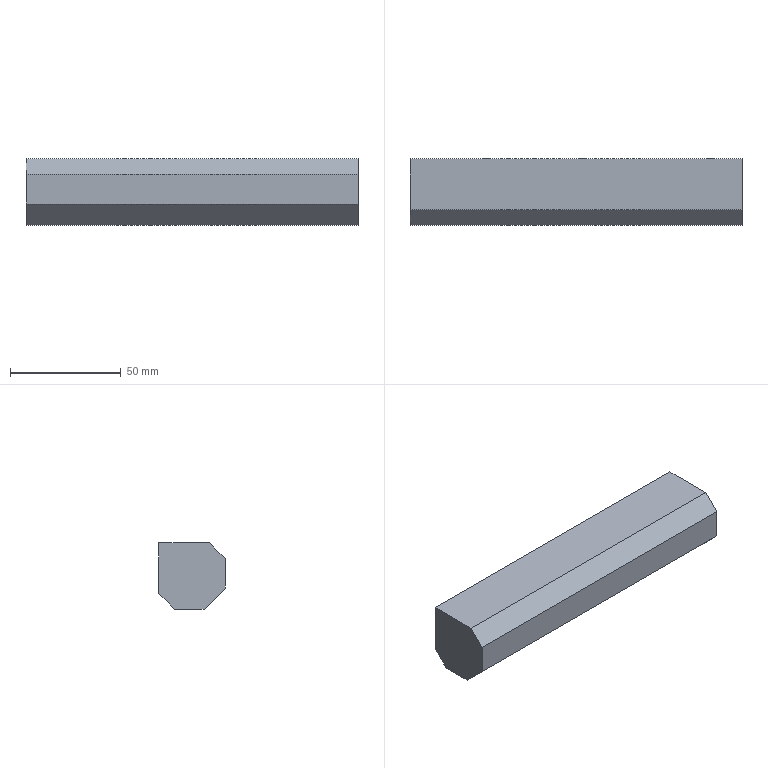Part | Mastercam | 1 solid | 18 faces | box 150 x 29.993 x 30 mm | volume 120343 mm3 | plane 12 | cylinder 6 | commonest cylinder face diameters 3.3 x6
STEP:
#1=CARTESIAN_POINT('',(0.,0.,0.));
#2=DIRECTION('',(0.,0.,1.));
#3=DIRECTION('',(1.,0.,0.));
#4=AXIS2_PLACEMENT_3D('',#1,#2,#3);
#5=CARTESIAN_POINT('',(97.5,23.7,-9.542));
#6=VERTEX_POINT('',#5);
#7=CARTESIAN_POINT('',(97.5,16.622,-16.62));
#8=VERTEX_POINT('',#7);
#9=CARTESIAN_POINT('',(97.5,26.528,-6.713));
#10=DIRECTION('',(0.,-0.7071,-0.7071));
#11=VECTOR('',#10,1.);
#12=LINE('',#9,#11);
#13=EDGE_CURVE('',#6,#8,#12,.T.);
#14=ORIENTED_EDGE('',*,*,#13,.T.);
#15=CARTESIAN_POINT('',(97.5,3.271,-16.62));
#16=VERTEX_POINT('',#15);
#17=CARTESIAN_POINT('',(97.5,0.,-16.62));
#18=DIRECTION('',(0.,1.,0.));
#19=VECTOR('',#18,1.);
#20=LINE('',#17,#19);
#21=EDGE_CURVE('',#16,#8,#20,.T.);
#22=ORIENTED_EDGE('',*,*,#21,.F.);
#23=CARTESIAN_POINT('',(97.5,-6.293,-7.056));
#24=VERTEX_POINT('',#23);
#25=CARTESIAN_POINT('',(97.5,-12.975,-0.3737));
#26=DIRECTION('',(0.,0.7071,-0.7071));
#27=VECTOR('',#26,1.);
#28=LINE('',#25,#27);
#29=EDGE_CURVE('',#24,#16,#28,.T.);
#30=ORIENTED_EDGE('',*,*,#29,.F.);
#31=CARTESIAN_POINT('',(97.5,-6.293,6.309));
#32=VERTEX_POINT('',#31);
#33=CARTESIAN_POINT('',(97.5,-6.293,0.));
#34=DIRECTION('',(0.,0.,-1.));
#35=VECTOR('',#34,1.);
#36=LINE('',#33,#35);
#37=EDGE_CURVE('',#32,#24,#36,.T.);
#38=ORIENTED_EDGE('',*,*,#37,.F.);
#39=CARTESIAN_POINT('',(97.5,0.7783,13.38));
#40=VERTEX_POINT('',#39);
#41=CARTESIAN_POINT('',(97.5,3.607,16.208));
#42=DIRECTION('',(0.,-0.7071,-0.7071));
#43=VECTOR('',#42,1.);
#44=LINE('',#41,#43);
#45=EDGE_CURVE('',#40,#32,#44,.T.);
#46=ORIENTED_EDGE('',*,*,#45,.F.);
#47=CARTESIAN_POINT('',(97.5,23.7,13.38));
#48=VERTEX_POINT('',#47);
#49=CARTESIAN_POINT('',(97.5,3.707,13.38));
#50=DIRECTION('',(0.,1.,0.));
#51=VECTOR('',#50,1.);
#52=LINE('',#49,#51);
#53=EDGE_CURVE('',#40,#48,#52,.T.);
#54=ORIENTED_EDGE('',*,*,#53,.T.);
#55=CARTESIAN_POINT('',(97.5,23.7,13.38));
#56=DIRECTION('',(0.,0.,-1.));
#57=VECTOR('',#56,1.);
#58=LINE('',#55,#57);
#59=EDGE_CURVE('',#48,#6,#58,.T.);
#60=ORIENTED_EDGE('',*,*,#59,.T.);
#61=EDGE_LOOP('',(#14,#22,#30,#38,#46,#54,#60));
#62=FACE_OUTER_BOUND('',#61,.T.);
#63=CARTESIAN_POINT('',(97.5,0.,0.));
#64=DIRECTION('',(1.,0.,0.));
#65=DIRECTION('',(0.,0.,-1.));
#66=AXIS2_PLACEMENT_3D('',#63,#64,#65);
#67=PLANE('',#66);
#68=ADVANCED_FACE('',(#62),#67,.F.);
#69=CARTESIAN_POINT('',(247.5,3.271,-16.62));
#70=VERTEX_POINT('',#69);
#71=CARTESIAN_POINT('',(247.5,16.622,-16.62));
#72=VERTEX_POINT('',#71);
#73=CARTESIAN_POINT('',(247.5,0.,-16.62));
#74=DIRECTION('',(0.,1.,0.));
#75=VECTOR('',#74,1.);
#76=LINE('',#73,#75);
#77=EDGE_CURVE('',#70,#72,#76,.T.);
#78=ORIENTED_EDGE('',*,*,#77,.T.);
#79=CARTESIAN_POINT('',(247.5,23.7,-9.542));
#80=VERTEX_POINT('',#79);
#81=CARTESIAN_POINT('',(247.5,26.528,-6.713));
#82=DIRECTION('',(0.,-0.7071,-0.7071));
#83=VECTOR('',#82,1.);
#84=LINE('',#81,#83);
#85=EDGE_CURVE('',#80,#72,#84,.T.);
#86=ORIENTED_EDGE('',*,*,#85,.F.);
#87=CARTESIAN_POINT('',(247.5,23.7,13.38));
#88=VERTEX_POINT('',#87);
#89=CARTESIAN_POINT('',(247.5,23.7,13.38));
#90=DIRECTION('',(0.,0.,-1.));
#91=VECTOR('',#90,1.);
#92=LINE('',#89,#91);
#93=EDGE_CURVE('',#88,#80,#92,.T.);
#94=ORIENTED_EDGE('',*,*,#93,.F.);
#95=CARTESIAN_POINT('',(247.5,0.7783,13.38));
#96=VERTEX_POINT('',#95);
#97=CARTESIAN_POINT('',(247.5,3.707,13.38));
#98=DIRECTION('',(0.,1.,0.));
#99=VECTOR('',#98,1.);
#100=LINE('',#97,#99);
#101=EDGE_CURVE('',#96,#88,#100,.T.);
#102=ORIENTED_EDGE('',*,*,#101,.F.);
#103=CARTESIAN_POINT('',(247.5,-6.293,6.309));
#104=VERTEX_POINT('',#103);
#105=CARTESIAN_POINT('',(247.5,3.607,16.208));
#106=DIRECTION('',(0.,-0.7071,-0.7071));
#107=VECTOR('',#106,1.);
#108=LINE('',#105,#107);
#109=EDGE_CURVE('',#96,#104,#108,.T.);
#110=ORIENTED_EDGE('',*,*,#109,.T.);
#111=CARTESIAN_POINT('',(247.5,-6.293,-7.056));
#112=VERTEX_POINT('',#111);
#113=CARTESIAN_POINT('',(247.5,-6.293,0.));
#114=DIRECTION('',(0.,0.,-1.));
#115=VECTOR('',#114,1.);
#116=LINE('',#113,#115);
#117=EDGE_CURVE('',#104,#112,#116,.T.);
#118=ORIENTED_EDGE('',*,*,#117,.T.);
#119=CARTESIAN_POINT('',(247.5,-12.975,-0.3737));
#120=DIRECTION('',(0.,0.7071,-0.7071));
#121=VECTOR('',#120,1.);
#122=LINE('',#119,#121);
#123=EDGE_CURVE('',#112,#70,#122,.T.);
#124=ORIENTED_EDGE('',*,*,#123,.T.);
#125=EDGE_LOOP('',(#78,#86,#94,#102,#110,#118,#124));
#126=FACE_OUTER_BOUND('',#125,.T.);
#127=CARTESIAN_POINT('',(247.5,0.,0.));
#128=DIRECTION('',(1.,0.,0.));
#129=DIRECTION('',(0.,0.,-1.));
#130=AXIS2_PLACEMENT_3D('',#127,#128,#129);
#131=PLANE('',#130);
#132=ADVANCED_FACE('',(#126),#131,.T.);
#133=ORIENTED_EDGE('',*,*,#21,.T.);
#134=CARTESIAN_POINT('',(97.5,16.622,-16.62));
#135=DIRECTION('',(1.,0.,0.));
#136=VECTOR('',#135,1.);
#137=LINE('',#134,#136);
#138=EDGE_CURVE('',#8,#72,#137,.T.);
#139=ORIENTED_EDGE('',*,*,#138,.T.);
#140=ORIENTED_EDGE('',*,*,#77,.F.);
#141=CARTESIAN_POINT('',(97.5,3.271,-16.62));
#142=DIRECTION('',(1.,0.,0.));
#143=VECTOR('',#142,1.);
#144=LINE('',#141,#143);
#145=EDGE_CURVE('',#16,#70,#144,.T.);
#146=ORIENTED_EDGE('',*,*,#145,.F.);
#147=EDGE_LOOP('',(#133,#139,#140,#146));
#148=FACE_OUTER_BOUND('',#147,.T.);
#149=CARTESIAN_POINT('',(97.5,3.707,-16.62));
#150=DIRECTION('',(0.,0.,-1.));
#151=DIRECTION('',(0.,1.,0.));
#152=AXIS2_PLACEMENT_3D('',#149,#150,#151);
#153=PLANE('',#152);
#154=ADVANCED_FACE('',(#148),#153,.T.);
#155=CARTESIAN_POINT('',(234.7,23.7,2.505));
#156=VERTEX_POINT('',#155);
#157=CARTESIAN_POINT('',(233.05,23.7,4.155));
#158=VERTEX_POINT('',#157);
#159=CARTESIAN_POINT('',(233.05,23.7,2.505));
#160=DIRECTION('',(0.,-1.,0.));
#161=DIRECTION('',(1.,0.,0.));
#162=AXIS2_PLACEMENT_3D('',#159,#160,#161);
#163=CIRCLE('',#162,1.65);
#164=EDGE_CURVE('',#156,#158,#163,.T.);
#165=ORIENTED_EDGE('',*,*,#164,.T.);
#166=CARTESIAN_POINT('',(233.05,23.7,0.855));
#167=VERTEX_POINT('',#166);
#168=CARTESIAN_POINT('',(233.05,23.7,2.505));
#169=DIRECTION('',(0.,-1.,0.));
#170=DIRECTION('',(1.,0.,0.));
#171=AXIS2_PLACEMENT_3D('',#168,#169,#170);
#172=CIRCLE('',#171,1.65);
#173=EDGE_CURVE('',#158,#167,#172,.T.);
#174=ORIENTED_EDGE('',*,*,#173,.T.);
#175=CARTESIAN_POINT('',(233.05,23.7,2.505));
#176=DIRECTION('',(0.,-1.,0.));
#177=DIRECTION('',(1.,0.,0.));
#178=AXIS2_PLACEMENT_3D('',#175,#176,#177);
#179=CIRCLE('',#178,1.65);
#180=EDGE_CURVE('',#167,#156,#179,.T.);
#181=ORIENTED_EDGE('',*,*,#180,.T.);
#182=EDGE_LOOP('',(#165,#174,#181));
#183=FACE_BOUND('',#182,.T.);
#184=CARTESIAN_POINT('',(177.1,23.7,2.505));
#185=VERTEX_POINT('',#184);
#186=CARTESIAN_POINT('',(175.45,23.7,4.155));
#187=VERTEX_POINT('',#186);
#188=CARTESIAN_POINT('',(175.45,23.7,2.505));
#189=DIRECTION('',(0.,-1.,0.));
#190=DIRECTION('',(1.,0.,0.));
#191=AXIS2_PLACEMENT_3D('',#188,#189,#190);
#192=CIRCLE('',#191,1.65);
#193=EDGE_CURVE('',#185,#187,#192,.T.);
#194=ORIENTED_EDGE('',*,*,#193,.T.);
#195=CARTESIAN_POINT('',(175.45,23.7,0.855));
#196=VERTEX_POINT('',#195);
#197=CARTESIAN_POINT('',(175.45,23.7,2.505));
#198=DIRECTION('',(0.,-1.,0.));
#199=DIRECTION('',(1.,0.,0.));
#200=AXIS2_PLACEMENT_3D('',#197,#198,#199);
#201=CIRCLE('',#200,1.65);
#202=EDGE_CURVE('',#187,#196,#201,.T.);
#203=ORIENTED_EDGE('',*,*,#202,.T.);
#204=CARTESIAN_POINT('',(175.45,23.7,2.505));
#205=DIRECTION('',(0.,-1.,0.));
#206=DIRECTION('',(1.,0.,0.));
#207=AXIS2_PLACEMENT_3D('',#204,#205,#206);
#208=CIRCLE('',#207,1.65);
#209=EDGE_CURVE('',#196,#185,#208,.T.);
#210=ORIENTED_EDGE('',*,*,#209,.T.);
#211=EDGE_LOOP('',(#194,#203,#210));
#212=FACE_BOUND('',#211,.T.);
#213=CARTESIAN_POINT('',(133.65,23.7,2.505));
#214=VERTEX_POINT('',#213);
#215=CARTESIAN_POINT('',(132.,23.7,4.155));
#216=VERTEX_POINT('',#215);
#217=CARTESIAN_POINT('',(132.,23.7,2.505));
#218=DIRECTION('',(0.,-1.,0.));
#219=DIRECTION('',(1.,0.,0.));
#220=AXIS2_PLACEMENT_3D('',#217,#218,#219);
#221=CIRCLE('',#220,1.65);
#222=EDGE_CURVE('',#214,#216,#221,.T.);
#223=ORIENTED_EDGE('',*,*,#222,.T.);
#224=CARTESIAN_POINT('',(132.,23.7,0.855));
#225=VERTEX_POINT('',#224);
#226=CARTESIAN_POINT('',(132.,23.7,2.505));
#227=DIRECTION('',(0.,-1.,0.));
#228=DIRECTION('',(1.,0.,0.));
#229=AXIS2_PLACEMENT_3D('',#226,#227,#228);
#230=CIRCLE('',#229,1.65);
#231=EDGE_CURVE('',#216,#225,#230,.T.);
#232=ORIENTED_EDGE('',*,*,#231,.T.);
#233=CARTESIAN_POINT('',(132.,23.7,2.505));
#234=DIRECTION('',(0.,-1.,0.));
#235=DIRECTION('',(1.,0.,0.));
#236=AXIS2_PLACEMENT_3D('',#233,#234,#235);
#237=CIRCLE('',#236,1.65);
#238=EDGE_CURVE('',#225,#214,#237,.T.);
#239=ORIENTED_EDGE('',*,*,#238,.T.);
#240=EDGE_LOOP('',(#223,#232,#239));
#241=FACE_BOUND('',#240,.T.);
#242=CARTESIAN_POINT('',(97.5,23.7,-9.542));
#243=DIRECTION('',(1.,0.,0.));
#244=VECTOR('',#243,1.);
#245=LINE('',#242,#244);
#246=EDGE_CURVE('',#6,#80,#245,.T.);
#247=ORIENTED_EDGE('',*,*,#246,.F.);
#248=ORIENTED_EDGE('',*,*,#59,.F.);
#249=CARTESIAN_POINT('',(97.5,23.7,13.38));
#250=DIRECTION('',(1.,0.,0.));
#251=VECTOR('',#250,1.);
#252=LINE('',#249,#251);
#253=EDGE_CURVE('',#48,#88,#252,.T.);
#254=ORIENTED_EDGE('',*,*,#253,.T.);
#255=ORIENTED_EDGE('',*,*,#93,.T.);
#256=EDGE_LOOP('',(#247,#248,#254,#255));
#257=FACE_OUTER_BOUND('',#256,.T.);
#258=CARTESIAN_POINT('',(97.5,23.7,13.38));
#259=DIRECTION('',(0.,-1.,0.));
#260=DIRECTION('',(0.,0.,-1.));
#261=AXIS2_PLACEMENT_3D('',#258,#259,#260);
#262=PLANE('',#261);
#263=ADVANCED_FACE('',(#183,#212,#241,#257),#262,.F.);
#264=CARTESIAN_POINT('',(97.5,-6.293,-7.056));
#265=DIRECTION('',(-1.,0.,0.));
#266=VECTOR('',#265,1.);
#267=LINE('',#264,#266);
#268=EDGE_CURVE('',#112,#24,#267,.T.);
#269=ORIENTED_EDGE('',*,*,#268,.F.);
#270=ORIENTED_EDGE('',*,*,#117,.F.);
#271=CARTESIAN_POINT('',(97.5,-6.293,6.309));
#272=DIRECTION('',(1.,0.,0.));
#273=VECTOR('',#272,1.);
#274=LINE('',#271,#273);
#275=EDGE_CURVE('',#32,#104,#274,.T.);
#276=ORIENTED_EDGE('',*,*,#275,.F.);
#277=ORIENTED_EDGE('',*,*,#37,.T.);
#278=EDGE_LOOP('',(#269,#270,#276,#277));
#279=FACE_OUTER_BOUND('',#278,.T.);
#280=CARTESIAN_POINT('',(97.5,-6.293,13.38));
#281=DIRECTION('',(0.,-1.,0.));
#282=DIRECTION('',(0.,0.,-1.));
#283=AXIS2_PLACEMENT_3D('',#280,#281,#282);
#284=PLANE('',#283);
#285=ADVANCED_FACE('',(#279),#284,.T.);
#286=ORIENTED_EDGE('',*,*,#53,.F.);
#287=CARTESIAN_POINT('',(97.5,0.7783,13.38));
#288=DIRECTION('',(1.,0.,0.));
#289=VECTOR('',#288,1.);
#290=LINE('',#287,#289);
#291=EDGE_CURVE('',#40,#96,#290,.T.);
#292=ORIENTED_EDGE('',*,*,#291,.T.);
#293=ORIENTED_EDGE('',*,*,#101,.T.);
#294=ORIENTED_EDGE('',*,*,#253,.F.);
#295=EDGE_LOOP('',(#286,#292,#293,#294));
#296=FACE_OUTER_BOUND('',#295,.T.);
#297=CARTESIAN_POINT('',(97.5,3.707,13.38));
#298=DIRECTION('',(0.,0.,-1.));
#299=DIRECTION('',(-1.,0.,0.));
#300=AXIS2_PLACEMENT_3D('',#297,#298,#299);
#301=PLANE('',#300);
#302=ADVANCED_FACE('',(#296),#301,.F.);
#303=CARTESIAN_POINT('',(132.,13.7,0.855));
#304=VERTEX_POINT('',#303);
#305=CARTESIAN_POINT('',(132.,13.7,0.855));
#306=DIRECTION('',(0.,1.,0.));
#307=VECTOR('',#306,1.);
#308=LINE('',#305,#307);
#309=EDGE_CURVE('',#304,#225,#308,.T.);
#310=ORIENTED_EDGE('',*,*,#309,.T.);
#311=ORIENTED_EDGE('',*,*,#231,.F.);
#312=CARTESIAN_POINT('',(132.,13.7,4.155));
#313=VERTEX_POINT('',#312);
#314=CARTESIAN_POINT('',(132.,13.7,4.155));
#315=DIRECTION('',(0.,1.,0.));
#316=VECTOR('',#315,1.);
#317=LINE('',#314,#316);
#318=EDGE_CURVE('',#313,#216,#317,.T.);
#319=ORIENTED_EDGE('',*,*,#318,.F.);
#320=CARTESIAN_POINT('',(132.,13.7,2.505));
#321=DIRECTION('',(0.,-1.,0.));
#322=DIRECTION('',(1.,0.,0.));
#323=AXIS2_PLACEMENT_3D('',#320,#321,#322);
#324=CIRCLE('',#323,1.65);
#325=EDGE_CURVE('',#313,#304,#324,.T.);
#326=ORIENTED_EDGE('',*,*,#325,.T.);
#327=EDGE_LOOP('',(#310,#311,#319,#326));
#328=FACE_OUTER_BOUND('',#327,.T.);
#329=CARTESIAN_POINT('',(132.,13.7,2.505));
#330=DIRECTION('',(0.,1.,0.));
#331=DIRECTION('',(1.,0.,0.));
#332=AXIS2_PLACEMENT_3D('',#329,#330,#331);
#333=CYLINDRICAL_SURFACE('',#332,1.65);
#334=ADVANCED_FACE('',(#328),#333,.F.);
#335=CARTESIAN_POINT('',(133.65,13.7,2.505));
#336=VERTEX_POINT('',#335);
#337=CARTESIAN_POINT('',(132.,13.7,2.505));
#338=DIRECTION('',(0.,-1.,0.));
#339=DIRECTION('',(1.,0.,0.));
#340=AXIS2_PLACEMENT_3D('',#337,#338,#339);
#341=CIRCLE('',#340,1.65);
#342=EDGE_CURVE('',#304,#336,#341,.T.);
#343=ORIENTED_EDGE('',*,*,#342,.F.);
#344=ORIENTED_EDGE('',*,*,#325,.F.);
#345=CARTESIAN_POINT('',(132.,13.7,2.505));
#346=DIRECTION('',(0.,-1.,0.));
#347=DIRECTION('',(1.,0.,0.));
#348=AXIS2_PLACEMENT_3D('',#345,#346,#347);
#349=CIRCLE('',#348,1.65);
#350=EDGE_CURVE('',#336,#313,#349,.T.);
#351=ORIENTED_EDGE('',*,*,#350,.F.);
#352=EDGE_LOOP('',(#343,#344,#351));
#353=FACE_OUTER_BOUND('',#352,.T.);
#354=CARTESIAN_POINT('',(132.,13.7,2.505));
#355=DIRECTION('',(0.,-1.,0.));
#356=DIRECTION('',(0.,0.,-1.));
#357=AXIS2_PLACEMENT_3D('',#354,#355,#356);
#358=PLANE('',#357);
#359=ADVANCED_FACE('',(#353),#358,.F.);
#360=CARTESIAN_POINT('',(175.45,13.7,0.855));
#361=VERTEX_POINT('',#360);
#362=CARTESIAN_POINT('',(175.45,13.7,0.855));
#363=DIRECTION('',(0.,1.,0.));
#364=VECTOR('',#363,1.);
#365=LINE('',#362,#364);
#366=EDGE_CURVE('',#361,#196,#365,.T.);
#367=ORIENTED_EDGE('',*,*,#366,.T.);
#368=ORIENTED_EDGE('',*,*,#202,.F.);
#369=CARTESIAN_POINT('',(175.45,13.7,4.155));
#370=VERTEX_POINT('',#369);
#371=CARTESIAN_POINT('',(175.45,13.7,4.155));
#372=DIRECTION('',(0.,1.,0.));
#373=VECTOR('',#372,1.);
#374=LINE('',#371,#373);
#375=EDGE_CURVE('',#370,#187,#374,.T.);
#376=ORIENTED_EDGE('',*,*,#375,.F.);
#377=CARTESIAN_POINT('',(175.45,13.7,2.505));
#378=DIRECTION('',(0.,-1.,0.));
#379=DIRECTION('',(1.,0.,0.));
#380=AXIS2_PLACEMENT_3D('',#377,#378,#379);
#381=CIRCLE('',#380,1.65);
#382=EDGE_CURVE('',#370,#361,#381,.T.);
#383=ORIENTED_EDGE('',*,*,#382,.T.);
#384=EDGE_LOOP('',(#367,#368,#376,#383));
#385=FACE_OUTER_BOUND('',#384,.T.);
#386=CARTESIAN_POINT('',(175.45,13.7,2.505));
#387=DIRECTION('',(0.,1.,0.));
#388=DIRECTION('',(1.,0.,0.));
#389=AXIS2_PLACEMENT_3D('',#386,#387,#388);
#390=CYLINDRICAL_SURFACE('',#389,1.65);
#391=ADVANCED_FACE('',(#385),#390,.F.);
#392=CARTESIAN_POINT('',(177.1,13.7,2.505));
#393=VERTEX_POINT('',#392);
#394=CARTESIAN_POINT('',(175.45,13.7,2.505));
#395=DIRECTION('',(0.,-1.,0.));
#396=DIRECTION('',(1.,0.,0.));
#397=AXIS2_PLACEMENT_3D('',#394,#395,#396);
#398=CIRCLE('',#397,1.65);
#399=EDGE_CURVE('',#361,#393,#398,.T.);
#400=ORIENTED_EDGE('',*,*,#399,.F.);
#401=ORIENTED_EDGE('',*,*,#382,.F.);
#402=CARTESIAN_POINT('',(175.45,13.7,2.505));
#403=DIRECTION('',(0.,-1.,0.));
#404=DIRECTION('',(1.,0.,0.));
#405=AXIS2_PLACEMENT_3D('',#402,#403,#404);
#406=CIRCLE('',#405,1.65);
#407=EDGE_CURVE('',#393,#370,#406,.T.);
#408=ORIENTED_EDGE('',*,*,#407,.F.);
#409=EDGE_LOOP('',(#400,#401,#408));
#410=FACE_OUTER_BOUND('',#409,.T.);
#411=CARTESIAN_POINT('',(175.45,13.7,2.505));
#412=DIRECTION('',(0.,-1.,0.));
#413=DIRECTION('',(0.,0.,-1.));
#414=AXIS2_PLACEMENT_3D('',#411,#412,#413);
#415=PLANE('',#414);
#416=ADVANCED_FACE('',(#410),#415,.F.);
#417=CARTESIAN_POINT('',(233.05,13.7,0.855));
#418=VERTEX_POINT('',#417);
#419=CARTESIAN_POINT('',(233.05,13.7,0.855));
#420=DIRECTION('',(0.,1.,0.));
#421=VECTOR('',#420,1.);
#422=LINE('',#419,#421);
#423=EDGE_CURVE('',#418,#167,#422,.T.);
#424=ORIENTED_EDGE('',*,*,#423,.T.);
#425=ORIENTED_EDGE('',*,*,#173,.F.);
#426=CARTESIAN_POINT('',(233.05,13.7,4.155));
#427=VERTEX_POINT('',#426);
#428=CARTESIAN_POINT('',(233.05,13.7,4.155));
#429=DIRECTION('',(0.,1.,0.));
#430=VECTOR('',#429,1.);
#431=LINE('',#428,#430);
#432=EDGE_CURVE('',#427,#158,#431,.T.);
#433=ORIENTED_EDGE('',*,*,#432,.F.);
#434=CARTESIAN_POINT('',(233.05,13.7,2.505));
#435=DIRECTION('',(0.,-1.,0.));
#436=DIRECTION('',(1.,0.,0.));
#437=AXIS2_PLACEMENT_3D('',#434,#435,#436);
#438=CIRCLE('',#437,1.65);
#439=EDGE_CURVE('',#427,#418,#438,.T.);
#440=ORIENTED_EDGE('',*,*,#439,.T.);
#441=EDGE_LOOP('',(#424,#425,#433,#440));
#442=FACE_OUTER_BOUND('',#441,.T.);
#443=CARTESIAN_POINT('',(233.05,13.7,2.505));
#444=DIRECTION('',(0.,1.,0.));
#445=DIRECTION('',(1.,0.,0.));
#446=AXIS2_PLACEMENT_3D('',#443,#444,#445);
#447=CYLINDRICAL_SURFACE('',#446,1.65);
#448=ADVANCED_FACE('',(#442),#447,.F.);
#449=CARTESIAN_POINT('',(234.7,13.7,2.505));
#450=VERTEX_POINT('',#449);
#451=CARTESIAN_POINT('',(233.05,13.7,2.505));
#452=DIRECTION('',(0.,-1.,0.));
#453=DIRECTION('',(1.,0.,0.));
#454=AXIS2_PLACEMENT_3D('',#451,#452,#453);
#455=CIRCLE('',#454,1.65);
#456=EDGE_CURVE('',#418,#450,#455,.T.);
#457=ORIENTED_EDGE('',*,*,#456,.F.);
#458=ORIENTED_EDGE('',*,*,#439,.F.);
#459=CARTESIAN_POINT('',(233.05,13.7,2.505));
#460=DIRECTION('',(0.,-1.,0.));
#461=DIRECTION('',(1.,0.,0.));
#462=AXIS2_PLACEMENT_3D('',#459,#460,#461);
#463=CIRCLE('',#462,1.65);
#464=EDGE_CURVE('',#450,#427,#463,.T.);
#465=ORIENTED_EDGE('',*,*,#464,.F.);
#466=EDGE_LOOP('',(#457,#458,#465));
#467=FACE_OUTER_BOUND('',#466,.T.);
#468=CARTESIAN_POINT('',(233.05,13.7,2.505));
#469=DIRECTION('',(0.,-1.,0.));
#470=DIRECTION('',(0.,0.,-1.));
#471=AXIS2_PLACEMENT_3D('',#468,#469,#470);
#472=PLANE('',#471);
#473=ADVANCED_FACE('',(#467),#472,.F.);
#474=ORIENTED_EDGE('',*,*,#275,.T.);
#475=ORIENTED_EDGE('',*,*,#109,.F.);
#476=ORIENTED_EDGE('',*,*,#291,.F.);
#477=ORIENTED_EDGE('',*,*,#45,.T.);
#478=EDGE_LOOP('',(#474,#475,#476,#477));
#479=FACE_OUTER_BOUND('',#478,.T.);
#480=CARTESIAN_POINT('',(247.5,3.607,16.208));
#481=DIRECTION('',(0.,0.7071,-0.7071));
#482=DIRECTION('',(0.,0.7071,0.7071));
#483=AXIS2_PLACEMENT_3D('',#480,#481,#482);
#484=PLANE('',#483);
#485=ADVANCED_FACE('',(#479),#484,.F.);
#486=ORIENTED_EDGE('',*,*,#145,.T.);
#487=ORIENTED_EDGE('',*,*,#123,.F.);
#488=ORIENTED_EDGE('',*,*,#268,.T.);
#489=ORIENTED_EDGE('',*,*,#29,.T.);
#490=EDGE_LOOP('',(#486,#487,#488,#489));
#491=FACE_OUTER_BOUND('',#490,.T.);
#492=CARTESIAN_POINT('',(247.5,-12.975,-0.3737));
#493=DIRECTION('',(0.,0.7071,0.7071));
#494=DIRECTION('',(0.,-0.7071,0.7071));
#495=AXIS2_PLACEMENT_3D('',#492,#493,#494);
#496=PLANE('',#495);
#497=ADVANCED_FACE('',(#491),#496,.F.);
#498=ORIENTED_EDGE('',*,*,#13,.F.);
#499=ORIENTED_EDGE('',*,*,#246,.T.);
#500=ORIENTED_EDGE('',*,*,#85,.T.);
#501=ORIENTED_EDGE('',*,*,#138,.F.);
#502=EDGE_LOOP('',(#498,#499,#500,#501));
#503=FACE_OUTER_BOUND('',#502,.T.);
#504=CARTESIAN_POINT('',(247.5,26.528,-6.713));
#505=DIRECTION('',(0.,0.7071,-0.7071));
#506=DIRECTION('',(0.,0.7071,0.7071));
#507=AXIS2_PLACEMENT_3D('',#504,#505,#506);
#508=PLANE('',#507);
#509=ADVANCED_FACE('',(#503),#508,.T.);
#510=ORIENTED_EDGE('',*,*,#309,.F.);
#511=ORIENTED_EDGE('',*,*,#342,.T.);
#512=ORIENTED_EDGE('',*,*,#350,.T.);
#513=ORIENTED_EDGE('',*,*,#318,.T.);
#514=ORIENTED_EDGE('',*,*,#222,.F.);
#515=ORIENTED_EDGE('',*,*,#238,.F.);
#516=EDGE_LOOP('',(#510,#511,#512,#513,#514,#515));
#517=FACE_OUTER_BOUND('',#516,.T.);
#518=CARTESIAN_POINT('',(132.,13.7,2.505));
#519=DIRECTION('',(0.,1.,0.));
#520=DIRECTION('',(-1.,0.,0.));
#521=AXIS2_PLACEMENT_3D('',#518,#519,#520);
#522=CYLINDRICAL_SURFACE('',#521,1.65);
#523=ADVANCED_FACE('',(#517),#522,.F.);
#524=ORIENTED_EDGE('',*,*,#366,.F.);
#525=ORIENTED_EDGE('',*,*,#399,.T.);
#526=ORIENTED_EDGE('',*,*,#407,.T.);
#527=ORIENTED_EDGE('',*,*,#375,.T.);
#528=ORIENTED_EDGE('',*,*,#193,.F.);
#529=ORIENTED_EDGE('',*,*,#209,.F.);
#530=EDGE_LOOP('',(#524,#525,#526,#527,#528,#529));
#531=FACE_OUTER_BOUND('',#530,.T.);
#532=CARTESIAN_POINT('',(175.45,13.7,2.505));
#533=DIRECTION('',(0.,1.,0.));
#534=DIRECTION('',(-1.,0.,0.));
#535=AXIS2_PLACEMENT_3D('',#532,#533,#534);
#536=CYLINDRICAL_SURFACE('',#535,1.65);
#537=ADVANCED_FACE('',(#531),#536,.F.);
#538=ORIENTED_EDGE('',*,*,#423,.F.);
#539=ORIENTED_EDGE('',*,*,#456,.T.);
#540=ORIENTED_EDGE('',*,*,#464,.T.);
#541=ORIENTED_EDGE('',*,*,#432,.T.);
#542=ORIENTED_EDGE('',*,*,#164,.F.);
#543=ORIENTED_EDGE('',*,*,#180,.F.);
#544=EDGE_LOOP('',(#538,#539,#540,#541,#542,#543));
#545=FACE_OUTER_BOUND('',#544,.T.);
#546=CARTESIAN_POINT('',(233.05,13.7,2.505));
#547=DIRECTION('',(0.,1.,0.));
#548=DIRECTION('',(-1.,0.,0.));
#549=AXIS2_PLACEMENT_3D('',#546,#547,#548);
#550=CYLINDRICAL_SURFACE('',#549,1.65);
#551=ADVANCED_FACE('',(#545),#550,.F.);
#552=CLOSED_SHELL('',(#68,#132,#154,#263,#285,#302,#334,#359,#391,#416,#448,#473,#485,#497,#509,#523,#537,#551));
#553=MANIFOLD_SOLID_BREP('',#552);
#554=(LENGTH_UNIT()NAMED_UNIT(*)SI_UNIT(.MILLI.,.METRE.));
#555=UNCERTAINTY_MEASURE_WITH_UNIT(LENGTH_MEASURE(0.005),#554,'','');
#556=(NAMED_UNIT(*)PLANE_ANGLE_UNIT()SI_UNIT($,.RADIAN.));
#557=(GEOMETRIC_REPRESENTATION_CONTEXT(3)GLOBAL_UNCERTAINTY_ASSIGNED_CONTEXT((#555))GLOBAL_UNIT_ASSIGNED_CONTEXT((#554,#556))REPRESENTATION_CONTEXT('',''));
#558=ADVANCED_BREP_SHAPE_REPRESENTATION('',(#4,#553),#557);